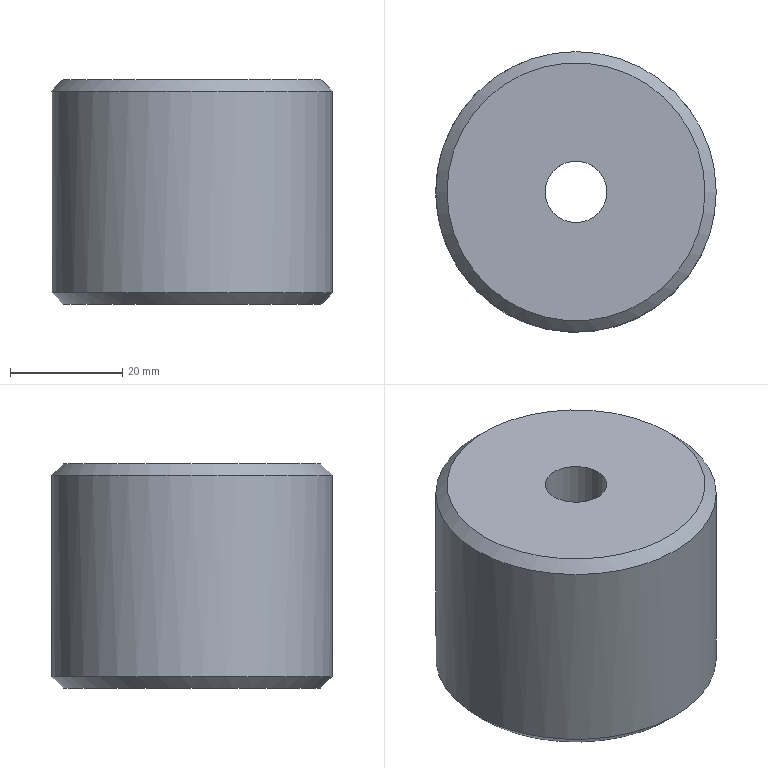Part | STEP file | gslz 2016.10.28-10_id2274_x_t | 1 solid | 8 faces | box 50 x 50 x 40 mm | volume 70960 mm3 | plane 3 | cylinder 3 | cone 2 | commonest cylinder face diameters 11 x1 17 x1 50 x1
STEP:
#1=CARTESIAN_POINT('',(0.,0.,0.));
#2=DIRECTION('',(0.,0.,1.));
#3=DIRECTION('',(1.,0.,0.));
#4=AXIS2_PLACEMENT_3D('',#1,#2,#3);
#5=CARTESIAN_POINT('',(456.5,225.,65.));
#6=VERTEX_POINT('',#5);
#7=CARTESIAN_POINT('',(433.5,225.,65.));
#8=DIRECTION('',(0.,0.,-1.));
#9=DIRECTION('',(1.,0.,0.));
#10=AXIS2_PLACEMENT_3D('',#7,#8,#9);
#11=CIRCLE('',#10,23.);
#12=CARTESIAN_POINT('',(433.5,225.,65.));
#13=DIRECTION('',(0.,0.,-1.));
#14=DIRECTION('',(-1.,0.,0.));
#15=AXIS2_PLACEMENT_3D('',#12,#13,#14);
#16=PLANE('',#15);
#17=CARTESIAN_POINT('',(0.,0.));
#18=DIRECTION('',(-1.,0.));
#19=AXIS2_PLACEMENT_2D('',#17,#18);
#20=CIRCLE('',#19,23.);
#21=(GEOMETRIC_REPRESENTATION_CONTEXT(2)PARAMETRIC_REPRESENTATION_CONTEXT()REPRESENTATION_CONTEXT('',''));
#22=DEFINITIONAL_REPRESENTATION('',(#20),#21);
#23=PCURVE('',#16,#22);
#24=CARTESIAN_POINT('',(433.5,225.,65.));
#25=DIRECTION('',(0.,0.,1.));
#26=DIRECTION('',(1.,0.,0.));
#27=AXIS2_PLACEMENT_3D('',#24,#25,#26);
#28=CONICAL_SURFACE('',#27,23.,0.7854);
#29=CARTESIAN_POINT('',(6.283,0.));
#30=DIRECTION('',(-1.,0.));
#31=VECTOR('',#30,1.);
#32=LINE('',#29,#31);
#33=(GEOMETRIC_REPRESENTATION_CONTEXT(2)PARAMETRIC_REPRESENTATION_CONTEXT()REPRESENTATION_CONTEXT('',''));
#34=DEFINITIONAL_REPRESENTATION('',(#32),#33);
#35=PCURVE('',#28,#34);
#36=SURFACE_CURVE('',#11,(#23,#35),.PCURVE_S1.);
#37=EDGE_CURVE('',#6,#6,#36,.T.);
#38=ORIENTED_EDGE('',*,*,#37,.T.);
#39=EDGE_LOOP('',(#38));
#40=FACE_BOUND('',#39,.T.);
#41=CARTESIAN_POINT('',(442.,225.,65.));
#42=VERTEX_POINT('',#41);
#43=CARTESIAN_POINT('',(433.5,225.,65.));
#44=DIRECTION('',(0.,0.,1.));
#45=DIRECTION('',(1.,0.,0.));
#46=AXIS2_PLACEMENT_3D('',#43,#44,#45);
#47=CIRCLE('',#46,8.5);
#48=CARTESIAN_POINT('',(-8.5,0.));
#49=CARTESIAN_POINT('',(-8.5,14.722));
#50=CARTESIAN_POINT('',(4.25,7.361));
#51=CARTESIAN_POINT('',(17.,0.));
#52=CARTESIAN_POINT('',(4.25,-7.361));
#53=CARTESIAN_POINT('',(-8.5,-14.722));
#54=CARTESIAN_POINT('',(-8.5,0.));
#55=(BOUNDED_CURVE()B_SPLINE_CURVE(2,(#48,#49,#50,#51,#52,#53,#54),.UNSPECIFIED.,.T.,.F.)B_SPLINE_CURVE_WITH_KNOTS((1,2,2,2,2,1),(-2.094,0.,2.094,4.189,6.283,8.378),.UNSPECIFIED.)CURVE()GEOMETRIC_REPRESENTATION_ITEM()RATIONAL_B_SPLINE_CURVE((1.,0.5,1.,0.5,1.,0.5,1.))REPRESENTATION_ITEM(''));
#56=(GEOMETRIC_REPRESENTATION_CONTEXT(2)PARAMETRIC_REPRESENTATION_CONTEXT()REPRESENTATION_CONTEXT('',''));
#57=DEFINITIONAL_REPRESENTATION('',(#55),#56);
#58=PCURVE('',#16,#57);
#59=CARTESIAN_POINT('',(433.5,225.,65.));
#60=DIRECTION('',(0.,0.,1.));
#61=DIRECTION('',(1.,0.,0.));
#62=AXIS2_PLACEMENT_3D('',#59,#60,#61);
#63=CYLINDRICAL_SURFACE('',#62,8.5);
#64=CARTESIAN_POINT('',(0.,0.));
#65=DIRECTION('',(1.,0.));
#66=VECTOR('',#65,1.);
#67=LINE('',#64,#66);
#68=(GEOMETRIC_REPRESENTATION_CONTEXT(2)PARAMETRIC_REPRESENTATION_CONTEXT()REPRESENTATION_CONTEXT('',''));
#69=DEFINITIONAL_REPRESENTATION('',(#67),#68);
#70=PCURVE('',#63,#69);
#71=SURFACE_CURVE('',#47,(#58,#70),.PCURVE_S1.);
#72=EDGE_CURVE('',#42,#42,#71,.T.);
#73=ORIENTED_EDGE('',*,*,#72,.T.);
#74=EDGE_LOOP('',(#73));
#75=FACE_BOUND('',#74,.T.);
#76=ADVANCED_FACE('',(#40,#75),#16,.T.);
#77=CARTESIAN_POINT('',(408.5,225.,103.));
#78=VERTEX_POINT('',#77);
#79=CARTESIAN_POINT('',(458.5,225.,103.));
#80=VERTEX_POINT('',#79);
#81=CARTESIAN_POINT('',(433.5,225.,103.));
#82=DIRECTION('',(0.,0.,-1.));
#83=DIRECTION('',(-1.,0.,0.));
#84=AXIS2_PLACEMENT_3D('',#81,#82,#83);
#85=CIRCLE('',#84,25.);
#86=CARTESIAN_POINT('',(433.5,225.,60.));
#87=DIRECTION('',(0.,0.,1.));
#88=DIRECTION('',(1.,0.,0.));
#89=AXIS2_PLACEMENT_3D('',#86,#87,#88);
#90=CYLINDRICAL_SURFACE('',#89,25.);
#91=CARTESIAN_POINT('',(3.142,43.));
#92=DIRECTION('',(-1.,0.));
#93=VECTOR('',#92,1.);
#94=LINE('',#91,#93);
#95=(GEOMETRIC_REPRESENTATION_CONTEXT(2)PARAMETRIC_REPRESENTATION_CONTEXT()REPRESENTATION_CONTEXT('',''));
#96=DEFINITIONAL_REPRESENTATION('',(#94),#95);
#97=PCURVE('',#90,#96);
#98=CARTESIAN_POINT('',(433.5,225.,103.));
#99=DIRECTION('',(0.,0.,-1.));
#100=DIRECTION('',(-1.,0.,0.));
#101=AXIS2_PLACEMENT_3D('',#98,#99,#100);
#102=CONICAL_SURFACE('',#101,25.,0.7854);
#103=CARTESIAN_POINT('',(0.,0.));
#104=DIRECTION('',(1.,0.));
#105=VECTOR('',#104,1.);
#106=LINE('',#103,#105);
#107=(GEOMETRIC_REPRESENTATION_CONTEXT(2)PARAMETRIC_REPRESENTATION_CONTEXT()REPRESENTATION_CONTEXT('',''));
#108=DEFINITIONAL_REPRESENTATION('',(#106),#107);
#109=PCURVE('',#102,#108);
#110=SURFACE_CURVE('',#85,(#97,#109),.PCURVE_S1.);
#111=EDGE_CURVE('',#78,#80,#110,.T.);
#112=ORIENTED_EDGE('',*,*,#111,.T.);
#113=CARTESIAN_POINT('',(458.5,225.,67.));
#114=VERTEX_POINT('',#113);
#115=CARTESIAN_POINT('',(458.5,225.,67.));
#116=CARTESIAN_POINT('',(458.5,225.,103.));
#117=B_SPLINE_CURVE_WITH_KNOTS('',1,(#115,#116),.UNSPECIFIED.,.F.,.F.,(2,2),(7.,43.),.PIECEWISE_BEZIER_KNOTS.);
#118=CARTESIAN_POINT('',(0.,0.));
#119=DIRECTION('',(0.,1.));
#120=VECTOR('',#119,1.);
#121=LINE('',#118,#120);
#122=(GEOMETRIC_REPRESENTATION_CONTEXT(2)PARAMETRIC_REPRESENTATION_CONTEXT()REPRESENTATION_CONTEXT('',''));
#123=DEFINITIONAL_REPRESENTATION('',(#121),#122);
#124=PCURVE('',#90,#123);
#125=CARTESIAN_POINT('',(6.283,0.));
#126=DIRECTION('',(0.,1.));
#127=VECTOR('',#126,1.);
#128=LINE('',#125,#127);
#129=(GEOMETRIC_REPRESENTATION_CONTEXT(2)PARAMETRIC_REPRESENTATION_CONTEXT()REPRESENTATION_CONTEXT('',''));
#130=DEFINITIONAL_REPRESENTATION('',(#128),#129);
#131=PCURVE('',#90,#130);
#132=SEAM_CURVE('',#117,(#124,#131),.PCURVE_S1.);
#133=EDGE_CURVE('',#114,#80,#132,.T.);
#134=ORIENTED_EDGE('',*,*,#133,.F.);
#135=CARTESIAN_POINT('',(433.5,225.,67.));
#136=DIRECTION('',(0.,0.,1.));
#137=DIRECTION('',(1.,0.,0.));
#138=AXIS2_PLACEMENT_3D('',#135,#136,#137);
#139=CIRCLE('',#138,25.);
#140=CARTESIAN_POINT('',(0.,7.));
#141=DIRECTION('',(1.,0.));
#142=VECTOR('',#141,1.);
#143=LINE('',#140,#142);
#144=(GEOMETRIC_REPRESENTATION_CONTEXT(2)PARAMETRIC_REPRESENTATION_CONTEXT()REPRESENTATION_CONTEXT('',''));
#145=DEFINITIONAL_REPRESENTATION('',(#143),#144);
#146=PCURVE('',#90,#145);
#147=CARTESIAN_POINT('',(0.,2.));
#148=DIRECTION('',(1.,0.));
#149=VECTOR('',#148,1.);
#150=LINE('',#147,#149);
#151=(GEOMETRIC_REPRESENTATION_CONTEXT(2)PARAMETRIC_REPRESENTATION_CONTEXT()REPRESENTATION_CONTEXT('',''));
#152=DEFINITIONAL_REPRESENTATION('',(#150),#151);
#153=PCURVE('',#28,#152);
#154=SURFACE_CURVE('',#139,(#146,#153),.PCURVE_S1.);
#155=EDGE_CURVE('',#114,#114,#154,.T.);
#156=ORIENTED_EDGE('',*,*,#155,.T.);
#157=ORIENTED_EDGE('',*,*,#133,.T.);
#158=CARTESIAN_POINT('',(433.5,225.,103.));
#159=DIRECTION('',(0.,0.,-1.));
#160=DIRECTION('',(-1.,0.,0.));
#161=AXIS2_PLACEMENT_3D('',#158,#159,#160);
#162=CIRCLE('',#161,25.);
#163=CARTESIAN_POINT('',(9.425,43.));
#164=DIRECTION('',(-1.,0.));
#165=VECTOR('',#164,1.);
#166=LINE('',#163,#165);
#167=(GEOMETRIC_REPRESENTATION_CONTEXT(2)PARAMETRIC_REPRESENTATION_CONTEXT()REPRESENTATION_CONTEXT('',''));
#168=DEFINITIONAL_REPRESENTATION('',(#166),#167);
#169=PCURVE('',#90,#168);
#170=CARTESIAN_POINT('',(0.,0.));
#171=DIRECTION('',(1.,0.));
#172=VECTOR('',#171,1.);
#173=LINE('',#170,#172);
#174=(GEOMETRIC_REPRESENTATION_CONTEXT(2)PARAMETRIC_REPRESENTATION_CONTEXT()REPRESENTATION_CONTEXT('',''));
#175=DEFINITIONAL_REPRESENTATION('',(#173),#174);
#176=PCURVE('',#102,#175);
#177=SURFACE_CURVE('',#162,(#169,#176),.PCURVE_S1.);
#178=EDGE_CURVE('',#80,#78,#177,.T.);
#179=ORIENTED_EDGE('',*,*,#178,.T.);
#180=EDGE_LOOP('',(#112,#134,#156,#157,#179));
#181=FACE_BOUND('',#180,.T.);
#182=ADVANCED_FACE('',(#181),#90,.T.);
#183=CARTESIAN_POINT('',(439.,225.,105.));
#184=VERTEX_POINT('',#183);
#185=CARTESIAN_POINT('',(428.,225.,105.));
#186=VERTEX_POINT('',#185);
#187=CARTESIAN_POINT('',(433.5,225.,105.));
#188=DIRECTION('',(0.,0.,1.));
#189=DIRECTION('',(-1.,0.,0.));
#190=AXIS2_PLACEMENT_3D('',#187,#188,#189);
#191=CIRCLE('',#190,5.5);
#192=CARTESIAN_POINT('',(433.5,225.,37.));
#193=DIRECTION('',(0.,0.,1.));
#194=DIRECTION('',(1.,0.,0.));
#195=AXIS2_PLACEMENT_3D('',#192,#193,#194);
#196=CYLINDRICAL_SURFACE('',#195,5.5);
#197=CARTESIAN_POINT('',(-3.142,68.));
#198=DIRECTION('',(1.,0.));
#199=VECTOR('',#198,1.);
#200=LINE('',#197,#199);
#201=(GEOMETRIC_REPRESENTATION_CONTEXT(2)PARAMETRIC_REPRESENTATION_CONTEXT()REPRESENTATION_CONTEXT('',''));
#202=DEFINITIONAL_REPRESENTATION('',(#200),#201);
#203=PCURVE('',#196,#202);
#204=CARTESIAN_POINT('',(485.611,-263.723,105.));
#205=DIRECTION('',(0.,0.,1.));
#206=DIRECTION('',(1.,0.,0.));
#207=AXIS2_PLACEMENT_3D('',#204,#205,#206);
#208=PLANE('',#207);
#209=CARTESIAN_POINT('',(-52.111,488.723));
#210=DIRECTION('',(-1.,0.));
#211=AXIS2_PLACEMENT_2D('',#209,#210);
#212=CIRCLE('',#211,5.5);
#213=(GEOMETRIC_REPRESENTATION_CONTEXT(2)PARAMETRIC_REPRESENTATION_CONTEXT()REPRESENTATION_CONTEXT('',''));
#214=DEFINITIONAL_REPRESENTATION('',(#212),#213);
#215=PCURVE('',#208,#214);
#216=SURFACE_CURVE('',#191,(#203,#215),.PCURVE_S1.);
#217=EDGE_CURVE('',#184,#186,#216,.T.);
#218=ORIENTED_EDGE('',*,*,#217,.F.);
#219=CARTESIAN_POINT('',(439.,225.,89.));
#220=VERTEX_POINT('',#219);
#221=CARTESIAN_POINT('',(439.,225.,89.));
#222=CARTESIAN_POINT('',(439.,225.,105.));
#223=B_SPLINE_CURVE_WITH_KNOTS('',1,(#221,#222),.UNSPECIFIED.,.F.,.F.,(2,2),(52.,68.),.PIECEWISE_BEZIER_KNOTS.);
#224=CARTESIAN_POINT('',(0.,0.));
#225=DIRECTION('',(0.,1.));
#226=VECTOR('',#225,1.);
#227=LINE('',#224,#226);
#228=(GEOMETRIC_REPRESENTATION_CONTEXT(2)PARAMETRIC_REPRESENTATION_CONTEXT()REPRESENTATION_CONTEXT('',''));
#229=DEFINITIONAL_REPRESENTATION('',(#227),#228);
#230=PCURVE('',#196,#229);
#231=CARTESIAN_POINT('',(6.283,0.));
#232=DIRECTION('',(0.,1.));
#233=VECTOR('',#232,1.);
#234=LINE('',#231,#233);
#235=(GEOMETRIC_REPRESENTATION_CONTEXT(2)PARAMETRIC_REPRESENTATION_CONTEXT()REPRESENTATION_CONTEXT('',''));
#236=DEFINITIONAL_REPRESENTATION('',(#234),#235);
#237=PCURVE('',#196,#236);
#238=SEAM_CURVE('',#223,(#230,#237),.PCURVE_S1.);
#239=EDGE_CURVE('',#220,#184,#238,.T.);
#240=ORIENTED_EDGE('',*,*,#239,.F.);
#241=CARTESIAN_POINT('',(433.5,225.,89.));
#242=DIRECTION('',(0.,0.,-1.));
#243=DIRECTION('',(1.,0.,0.));
#244=AXIS2_PLACEMENT_3D('',#241,#242,#243);
#245=CIRCLE('',#244,5.5);
#246=CARTESIAN_POINT('',(6.283,52.));
#247=DIRECTION('',(-1.,0.));
#248=VECTOR('',#247,1.);
#249=LINE('',#246,#248);
#250=(GEOMETRIC_REPRESENTATION_CONTEXT(2)PARAMETRIC_REPRESENTATION_CONTEXT()REPRESENTATION_CONTEXT('',''));
#251=DEFINITIONAL_REPRESENTATION('',(#249),#250);
#252=PCURVE('',#196,#251);
#253=CARTESIAN_POINT('',(433.5,225.,89.));
#254=DIRECTION('',(0.,0.,-1.));
#255=DIRECTION('',(-1.,0.,0.));
#256=AXIS2_PLACEMENT_3D('',#253,#254,#255);
#257=PLANE('',#256);
#258=CARTESIAN_POINT('',(0.,0.));
#259=DIRECTION('',(-1.,0.));
#260=AXIS2_PLACEMENT_2D('',#258,#259);
#261=CIRCLE('',#260,5.5);
#262=(GEOMETRIC_REPRESENTATION_CONTEXT(2)PARAMETRIC_REPRESENTATION_CONTEXT()REPRESENTATION_CONTEXT('',''));
#263=DEFINITIONAL_REPRESENTATION('',(#261),#262);
#264=PCURVE('',#257,#263);
#265=SURFACE_CURVE('',#245,(#252,#264),.PCURVE_S1.);
#266=EDGE_CURVE('',#220,#220,#265,.T.);
#267=ORIENTED_EDGE('',*,*,#266,.F.);
#268=ORIENTED_EDGE('',*,*,#239,.T.);
#269=CARTESIAN_POINT('',(433.5,225.,105.));
#270=DIRECTION('',(0.,0.,1.));
#271=DIRECTION('',(-1.,0.,0.));
#272=AXIS2_PLACEMENT_3D('',#269,#270,#271);
#273=CIRCLE('',#272,5.5);
#274=CARTESIAN_POINT('',(3.142,68.));
#275=DIRECTION('',(1.,0.));
#276=VECTOR('',#275,1.);
#277=LINE('',#274,#276);
#278=(GEOMETRIC_REPRESENTATION_CONTEXT(2)PARAMETRIC_REPRESENTATION_CONTEXT()REPRESENTATION_CONTEXT('',''));
#279=DEFINITIONAL_REPRESENTATION('',(#277),#278);
#280=PCURVE('',#196,#279);
#281=CARTESIAN_POINT('',(-52.111,488.723));
#282=DIRECTION('',(-1.,0.));
#283=AXIS2_PLACEMENT_2D('',#281,#282);
#284=CIRCLE('',#283,5.5);
#285=(GEOMETRIC_REPRESENTATION_CONTEXT(2)PARAMETRIC_REPRESENTATION_CONTEXT()REPRESENTATION_CONTEXT('',''));
#286=DEFINITIONAL_REPRESENTATION('',(#284),#285);
#287=PCURVE('',#208,#286);
#288=SURFACE_CURVE('',#273,(#280,#287),.PCURVE_S1.);
#289=EDGE_CURVE('',#186,#184,#288,.T.);
#290=ORIENTED_EDGE('',*,*,#289,.F.);
#291=EDGE_LOOP('',(#218,#240,#267,#268,#290));
#292=FACE_BOUND('',#291,.F.);
#293=ADVANCED_FACE('',(#292),#196,.F.);
#294=CARTESIAN_POINT('',(410.5,225.,105.));
#295=VERTEX_POINT('',#294);
#296=CARTESIAN_POINT('',(433.5,225.,105.));
#297=DIRECTION('',(0.,0.,1.));
#298=DIRECTION('',(-1.,0.,0.));
#299=AXIS2_PLACEMENT_3D('',#296,#297,#298);
#300=CIRCLE('',#299,23.);
#301=CARTESIAN_POINT('',(-52.111,488.723));
#302=DIRECTION('',(-1.,0.));
#303=AXIS2_PLACEMENT_2D('',#301,#302);
#304=CIRCLE('',#303,23.);
#305=(GEOMETRIC_REPRESENTATION_CONTEXT(2)PARAMETRIC_REPRESENTATION_CONTEXT()REPRESENTATION_CONTEXT('',''));
#306=DEFINITIONAL_REPRESENTATION('',(#304),#305);
#307=PCURVE('',#208,#306);
#308=CARTESIAN_POINT('',(6.283,-2.));
#309=DIRECTION('',(-1.,0.));
#310=VECTOR('',#309,1.);
#311=LINE('',#308,#310);
#312=(GEOMETRIC_REPRESENTATION_CONTEXT(2)PARAMETRIC_REPRESENTATION_CONTEXT()REPRESENTATION_CONTEXT('',''));
#313=DEFINITIONAL_REPRESENTATION('',(#311),#312);
#314=PCURVE('',#102,#313);
#315=SURFACE_CURVE('',#300,(#307,#314),.PCURVE_S1.);
#316=EDGE_CURVE('',#295,#295,#315,.T.);
#317=ORIENTED_EDGE('',*,*,#316,.T.);
#318=EDGE_LOOP('',(#317));
#319=FACE_BOUND('',#318,.T.);
#320=ORIENTED_EDGE('',*,*,#289,.F.);
#321=ORIENTED_EDGE('',*,*,#217,.F.);
#322=EDGE_LOOP('',(#320,#321));
#323=FACE_BOUND('',#322,.T.);
#324=ADVANCED_FACE('',(#319,#323),#208,.T.);
#325=CARTESIAN_POINT('',(442.,225.,89.));
#326=VERTEX_POINT('',#325);
#327=CARTESIAN_POINT('',(433.5,225.,89.));
#328=DIRECTION('',(0.,0.,-1.));
#329=DIRECTION('',(1.,0.,0.));
#330=AXIS2_PLACEMENT_3D('',#327,#328,#329);
#331=CIRCLE('',#330,8.5);
#332=CARTESIAN_POINT('',(0.,0.));
#333=DIRECTION('',(-1.,0.));
#334=AXIS2_PLACEMENT_2D('',#332,#333);
#335=CIRCLE('',#334,8.5);
#336=(GEOMETRIC_REPRESENTATION_CONTEXT(2)PARAMETRIC_REPRESENTATION_CONTEXT()REPRESENTATION_CONTEXT('',''));
#337=DEFINITIONAL_REPRESENTATION('',(#335),#336);
#338=PCURVE('',#257,#337);
#339=CARTESIAN_POINT('',(6.283,24.));
#340=DIRECTION('',(-1.,0.));
#341=VECTOR('',#340,1.);
#342=LINE('',#339,#341);
#343=(GEOMETRIC_REPRESENTATION_CONTEXT(2)PARAMETRIC_REPRESENTATION_CONTEXT()REPRESENTATION_CONTEXT('',''));
#344=DEFINITIONAL_REPRESENTATION('',(#342),#343);
#345=PCURVE('',#63,#344);
#346=SURFACE_CURVE('',#331,(#338,#345),.PCURVE_S1.);
#347=EDGE_CURVE('',#326,#326,#346,.T.);
#348=ORIENTED_EDGE('',*,*,#347,.T.);
#349=EDGE_LOOP('',(#348));
#350=FACE_BOUND('',#349,.T.);
#351=ORIENTED_EDGE('',*,*,#266,.F.);
#352=EDGE_LOOP('',(#351));
#353=FACE_BOUND('',#352,.T.);
#354=ADVANCED_FACE('',(#350,#353),#257,.T.);
#355=ORIENTED_EDGE('',*,*,#72,.T.);
#356=CARTESIAN_POINT('',(442.,225.,65.));
#357=CARTESIAN_POINT('',(442.,225.,89.));
#358=B_SPLINE_CURVE_WITH_KNOTS('',1,(#356,#357),.UNSPECIFIED.,.F.,.F.,(2,2),(0.,24.),.PIECEWISE_BEZIER_KNOTS.);
#359=CARTESIAN_POINT('',(6.283,0.));
#360=DIRECTION('',(0.,1.));
#361=VECTOR('',#360,1.);
#362=LINE('',#359,#361);
#363=(GEOMETRIC_REPRESENTATION_CONTEXT(2)PARAMETRIC_REPRESENTATION_CONTEXT()REPRESENTATION_CONTEXT('',''));
#364=DEFINITIONAL_REPRESENTATION('',(#362),#363);
#365=PCURVE('',#63,#364);
#366=CARTESIAN_POINT('',(0.,0.));
#367=DIRECTION('',(0.,1.));
#368=VECTOR('',#367,1.);
#369=LINE('',#366,#368);
#370=(GEOMETRIC_REPRESENTATION_CONTEXT(2)PARAMETRIC_REPRESENTATION_CONTEXT()REPRESENTATION_CONTEXT('',''));
#371=DEFINITIONAL_REPRESENTATION('',(#369),#370);
#372=PCURVE('',#63,#371);
#373=SEAM_CURVE('',#358,(#365,#372),.PCURVE_S1.);
#374=EDGE_CURVE('',#42,#326,#373,.T.);
#375=ORIENTED_EDGE('',*,*,#374,.T.);
#376=ORIENTED_EDGE('',*,*,#347,.T.);
#377=ORIENTED_EDGE('',*,*,#374,.F.);
#378=EDGE_LOOP('',(#355,#375,#376,#377));
#379=FACE_BOUND('',#378,.F.);
#380=ADVANCED_FACE('',(#379),#63,.F.);
#381=ORIENTED_EDGE('',*,*,#316,.F.);
#382=CARTESIAN_POINT('',(410.5,225.,105.));
#383=CARTESIAN_POINT('',(408.5,225.,103.));
#384=B_SPLINE_CURVE_WITH_KNOTS('',1,(#382,#383),.UNSPECIFIED.,.F.,.F.,(2,2),(-2.828,0.),.PIECEWISE_BEZIER_KNOTS.);
#385=CARTESIAN_POINT('',(6.283,0.));
#386=DIRECTION('',(0.,1.));
#387=VECTOR('',#386,1.);
#388=LINE('',#385,#387);
#389=(GEOMETRIC_REPRESENTATION_CONTEXT(2)PARAMETRIC_REPRESENTATION_CONTEXT()REPRESENTATION_CONTEXT('',''));
#390=DEFINITIONAL_REPRESENTATION('',(#388),#389);
#391=PCURVE('',#102,#390);
#392=CARTESIAN_POINT('',(0.,0.));
#393=DIRECTION('',(0.,1.));
#394=VECTOR('',#393,1.);
#395=LINE('',#392,#394);
#396=(GEOMETRIC_REPRESENTATION_CONTEXT(2)PARAMETRIC_REPRESENTATION_CONTEXT()REPRESENTATION_CONTEXT('',''));
#397=DEFINITIONAL_REPRESENTATION('',(#395),#396);
#398=PCURVE('',#102,#397);
#399=SEAM_CURVE('',#384,(#391,#398),.PCURVE_S1.);
#400=EDGE_CURVE('',#295,#78,#399,.T.);
#401=ORIENTED_EDGE('',*,*,#400,.T.);
#402=ORIENTED_EDGE('',*,*,#178,.F.);
#403=ORIENTED_EDGE('',*,*,#111,.F.);
#404=ORIENTED_EDGE('',*,*,#400,.F.);
#405=EDGE_LOOP('',(#381,#401,#402,#403,#404));
#406=FACE_BOUND('',#405,.T.);
#407=ADVANCED_FACE('',(#406),#102,.T.);
#408=ORIENTED_EDGE('',*,*,#155,.F.);
#409=CARTESIAN_POINT('',(456.5,225.,65.));
#410=CARTESIAN_POINT('',(458.5,225.,67.));
#411=B_SPLINE_CURVE_WITH_KNOTS('',1,(#409,#410),.UNSPECIFIED.,.F.,.F.,(2,2),(0.,2.828),.PIECEWISE_BEZIER_KNOTS.);
#412=CARTESIAN_POINT('',(0.,0.));
#413=DIRECTION('',(0.,1.));
#414=VECTOR('',#413,1.);
#415=LINE('',#412,#414);
#416=(GEOMETRIC_REPRESENTATION_CONTEXT(2)PARAMETRIC_REPRESENTATION_CONTEXT()REPRESENTATION_CONTEXT('',''));
#417=DEFINITIONAL_REPRESENTATION('',(#415),#416);
#418=PCURVE('',#28,#417);
#419=CARTESIAN_POINT('',(6.283,0.));
#420=DIRECTION('',(0.,1.));
#421=VECTOR('',#420,1.);
#422=LINE('',#419,#421);
#423=(GEOMETRIC_REPRESENTATION_CONTEXT(2)PARAMETRIC_REPRESENTATION_CONTEXT()REPRESENTATION_CONTEXT('',''));
#424=DEFINITIONAL_REPRESENTATION('',(#422),#423);
#425=PCURVE('',#28,#424);
#426=SEAM_CURVE('',#411,(#418,#425),.PCURVE_S1.);
#427=EDGE_CURVE('',#6,#114,#426,.T.);
#428=ORIENTED_EDGE('',*,*,#427,.F.);
#429=ORIENTED_EDGE('',*,*,#37,.F.);
#430=ORIENTED_EDGE('',*,*,#427,.T.);
#431=EDGE_LOOP('',(#408,#428,#429,#430));
#432=FACE_BOUND('',#431,.T.);
#433=ADVANCED_FACE('',(#432),#28,.T.);
#434=CLOSED_SHELL('',(#76,#182,#293,#324,#354,#380,#407,#433));
#435=MANIFOLD_SOLID_BREP('',#434);
#436=(LENGTH_UNIT()NAMED_UNIT(*)SI_UNIT(.MILLI.,.METRE.));
#437=UNCERTAINTY_MEASURE_WITH_UNIT(LENGTH_MEASURE(0.00001),#436,'','');
#438=(NAMED_UNIT(*)PLANE_ANGLE_UNIT()SI_UNIT($,.RADIAN.));
#439=(NAMED_UNIT(*)SI_UNIT($,.STERADIAN.)SOLID_ANGLE_UNIT());
#440=(GEOMETRIC_REPRESENTATION_CONTEXT(3)GLOBAL_UNCERTAINTY_ASSIGNED_CONTEXT((#437))GLOBAL_UNIT_ASSIGNED_CONTEXT((#436,#438,#439))REPRESENTATION_CONTEXT('',''));
#441=ADVANCED_BREP_SHAPE_REPRESENTATION('',(#4,#435),#440);